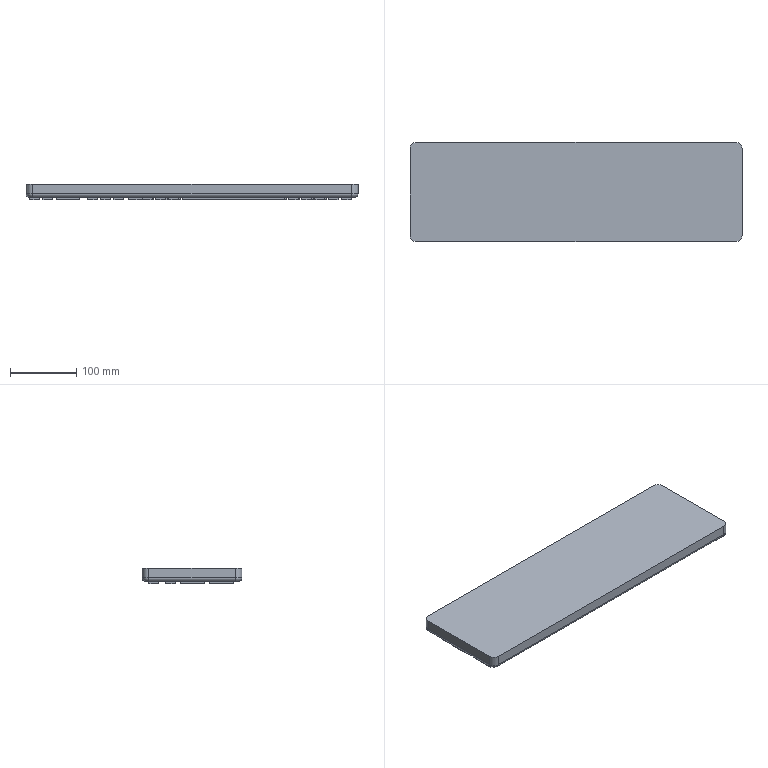Part | SolidWorks | features ICE 6, Fillet 2, Extrusion 1 | 1 solid | 624 faces | box 500 x 150 x 24 mm | volume 1615736 mm3 | plane 606 | cylinder 14 | torus 4 | commonest cylinder face diameters 4 x6 10 x4 20 x4